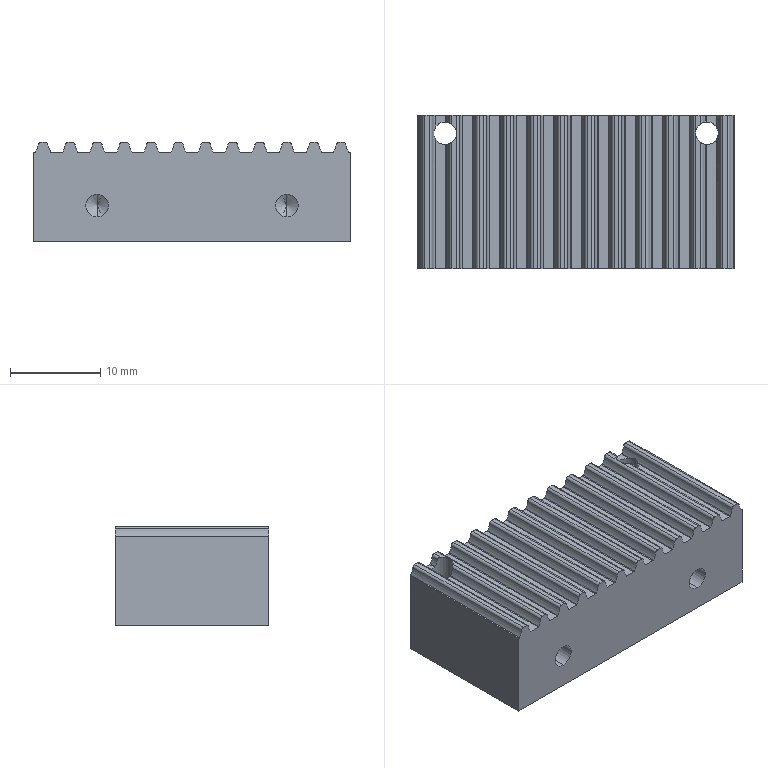Part | STEP file | 02-17 timing belt fixing block | 1 solid | 125 faces | box 35 x 17 x 11 mm | volume 5983 mm3 | cylinder 88 | plane 33 | cone 4 | commonest cylinder face diameters 0.2 x28 0.6 x26 3.9 x26 2.5 x8